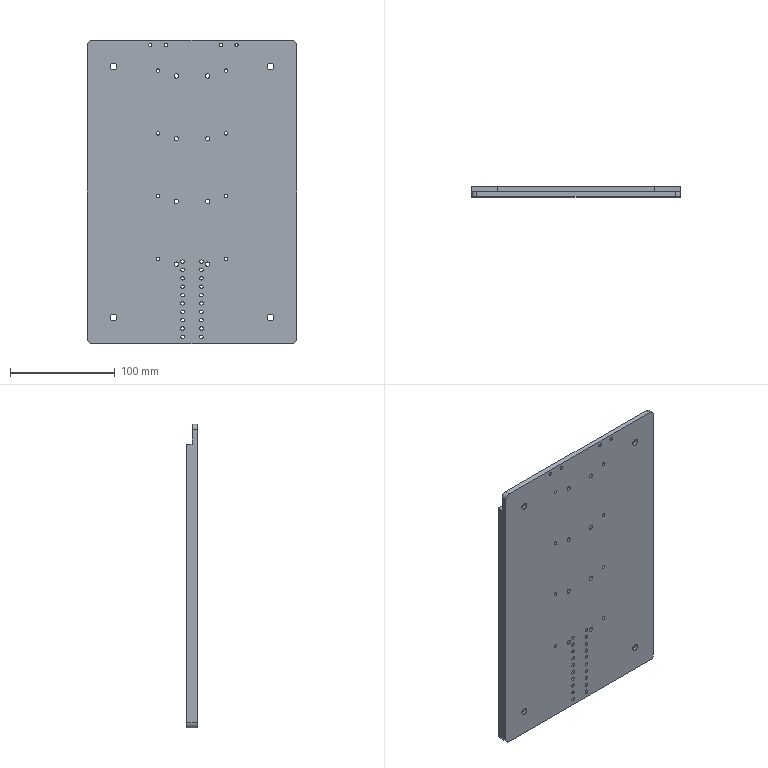Part | STEP file | 0-19-09 Discharge platform 1 | 1 solid | 112 faces | box 200 x 10 x 290 mm | volume 554142 mm3 | cylinder 100 | plane 12 | commonest cylinder face diameters 3.3 x64 4.2 x16 6.6 x8 11 x8 10 x4